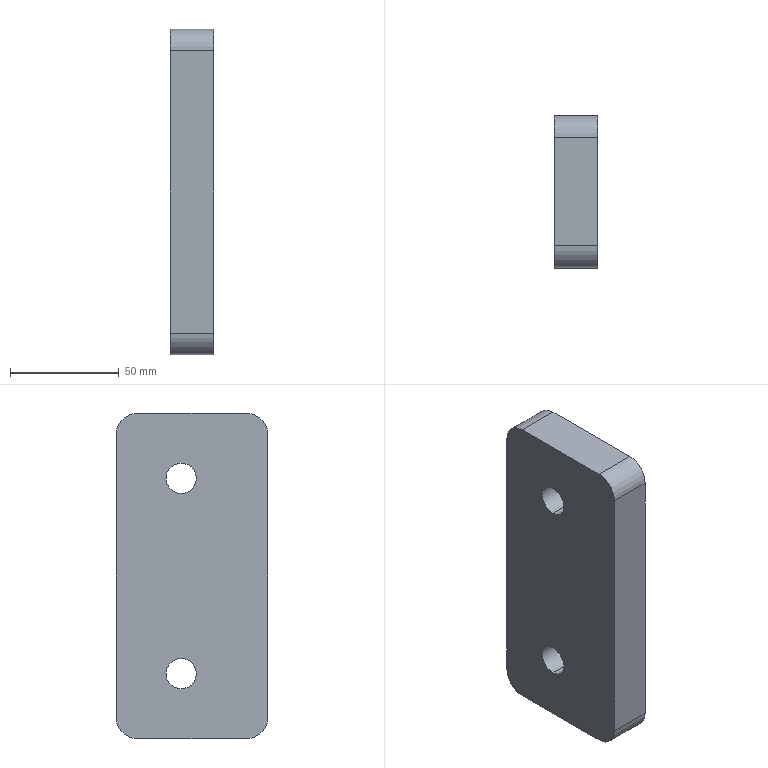Part | SolidWorks | 1 solid | 14 faces | box 20 x 70 x 150 mm | volume 202126 mm3 | cylinder 8 | plane 6 | commonest cylinder face diameters 14 x4 20 x4
STEP:
#1=CARTESIAN_POINT('',(-20.,5.,-38.));
#2=VERTEX_POINT('',#1);
#3=CARTESIAN_POINT('',(-20.,5.,-52.));
#4=VERTEX_POINT('',#3);
#5=CARTESIAN_POINT('',(-20.,5.,-45.));
#6=DIRECTION('',(-1.,0.,0.));
#7=DIRECTION('',(0.,0.,1.));
#8=AXIS2_PLACEMENT_3D('',#5,#6,#7);
#9=CIRCLE('',#8,7.);
#10=EDGE_CURVE('',#2,#4,#9,.T.);
#11=ORIENTED_EDGE('',*,*,#10,.T.);
#12=CARTESIAN_POINT('',(0.,5.,-52.));
#13=VERTEX_POINT('',#12);
#14=CARTESIAN_POINT('',(0.,5.,-52.));
#15=DIRECTION('',(1.,0.,0.));
#16=VECTOR('',#15,1000.);
#17=LINE('',#14,#16);
#18=EDGE_CURVE('',#4,#13,#17,.T.);
#19=ORIENTED_EDGE('',*,*,#18,.T.);
#20=CARTESIAN_POINT('',(0.,5.,-38.));
#21=VERTEX_POINT('',#20);
#22=CARTESIAN_POINT('',(0.,5.,-45.));
#23=DIRECTION('',(-1.,0.,0.));
#24=DIRECTION('',(0.,0.,1.));
#25=AXIS2_PLACEMENT_3D('',#22,#23,#24);
#26=CIRCLE('',#25,7.);
#27=EDGE_CURVE('',#21,#13,#26,.T.);
#28=ORIENTED_EDGE('',*,*,#27,.F.);
#29=CARTESIAN_POINT('',(0.,5.,-38.));
#30=DIRECTION('',(1.,0.,0.));
#31=VECTOR('',#30,1000.);
#32=LINE('',#29,#31);
#33=EDGE_CURVE('',#2,#21,#32,.T.);
#34=ORIENTED_EDGE('',*,*,#33,.F.);
#35=EDGE_LOOP('',(#11,#19,#28,#34));
#36=FACE_OUTER_BOUND('',#35,.T.);
#37=CARTESIAN_POINT('',(0.,5.,-45.));
#38=DIRECTION('',(1.,0.,0.));
#39=DIRECTION('',(0.,0.,1.));
#40=AXIS2_PLACEMENT_3D('',#37,#38,#39);
#41=CYLINDRICAL_SURFACE('',#40,7.);
#42=ADVANCED_FACE('',(#36),#41,.F.);
#43=CARTESIAN_POINT('',(-20.,5.,52.));
#44=VERTEX_POINT('',#43);
#45=CARTESIAN_POINT('',(-20.,5.,38.));
#46=VERTEX_POINT('',#45);
#47=CARTESIAN_POINT('',(-20.,5.,45.));
#48=DIRECTION('',(-1.,0.,0.));
#49=DIRECTION('',(0.,0.,1.));
#50=AXIS2_PLACEMENT_3D('',#47,#48,#49);
#51=CIRCLE('',#50,7.);
#52=EDGE_CURVE('',#44,#46,#51,.T.);
#53=ORIENTED_EDGE('',*,*,#52,.T.);
#54=CARTESIAN_POINT('',(0.,5.,38.));
#55=VERTEX_POINT('',#54);
#56=CARTESIAN_POINT('',(0.,5.,38.));
#57=DIRECTION('',(1.,0.,0.));
#58=VECTOR('',#57,1000.);
#59=LINE('',#56,#58);
#60=EDGE_CURVE('',#46,#55,#59,.T.);
#61=ORIENTED_EDGE('',*,*,#60,.T.);
#62=CARTESIAN_POINT('',(0.,5.,52.));
#63=VERTEX_POINT('',#62);
#64=CARTESIAN_POINT('',(0.,5.,45.));
#65=DIRECTION('',(-1.,0.,0.));
#66=DIRECTION('',(0.,0.,1.));
#67=AXIS2_PLACEMENT_3D('',#64,#65,#66);
#68=CIRCLE('',#67,7.);
#69=EDGE_CURVE('',#63,#55,#68,.T.);
#70=ORIENTED_EDGE('',*,*,#69,.F.);
#71=CARTESIAN_POINT('',(0.,5.,52.));
#72=DIRECTION('',(1.,0.,0.));
#73=VECTOR('',#72,1000.);
#74=LINE('',#71,#73);
#75=EDGE_CURVE('',#44,#63,#74,.T.);
#76=ORIENTED_EDGE('',*,*,#75,.F.);
#77=EDGE_LOOP('',(#53,#61,#70,#76));
#78=FACE_OUTER_BOUND('',#77,.T.);
#79=CARTESIAN_POINT('',(0.,5.,45.));
#80=DIRECTION('',(1.,0.,0.));
#81=DIRECTION('',(0.,0.,1.));
#82=AXIS2_PLACEMENT_3D('',#79,#80,#81);
#83=CYLINDRICAL_SURFACE('',#82,7.);
#84=ADVANCED_FACE('',(#78),#83,.F.);
#85=CARTESIAN_POINT('',(0.,25.,-75.));
#86=VERTEX_POINT('',#85);
#87=CARTESIAN_POINT('',(0.,-25.,-75.));
#88=VERTEX_POINT('',#87);
#89=CARTESIAN_POINT('',(0.,-35.,-75.));
#90=DIRECTION('',(0.,-1.,0.));
#91=VECTOR('',#90,1000.);
#92=LINE('',#89,#91);
#93=EDGE_CURVE('',#86,#88,#92,.T.);
#94=ORIENTED_EDGE('',*,*,#93,.T.);
#95=CARTESIAN_POINT('',(-20.,-25.,-75.));
#96=VERTEX_POINT('',#95);
#97=CARTESIAN_POINT('',(-20.,-25.,-75.));
#98=DIRECTION('',(1.,0.,0.));
#99=VECTOR('',#98,1000.);
#100=LINE('',#97,#99);
#101=EDGE_CURVE('',#96,#88,#100,.T.);
#102=ORIENTED_EDGE('',*,*,#101,.F.);
#103=CARTESIAN_POINT('',(-20.,25.,-75.));
#104=VERTEX_POINT('',#103);
#105=CARTESIAN_POINT('',(-20.,-35.,-75.));
#106=DIRECTION('',(0.,-1.,0.));
#107=VECTOR('',#106,1000.);
#108=LINE('',#105,#107);
#109=EDGE_CURVE('',#104,#96,#108,.T.);
#110=ORIENTED_EDGE('',*,*,#109,.F.);
#111=CARTESIAN_POINT('',(-20.,25.,-75.));
#112=DIRECTION('',(-1.,0.,0.));
#113=VECTOR('',#112,1000.);
#114=LINE('',#111,#113);
#115=EDGE_CURVE('',#86,#104,#114,.T.);
#116=ORIENTED_EDGE('',*,*,#115,.F.);
#117=EDGE_LOOP('',(#94,#102,#110,#116));
#118=FACE_OUTER_BOUND('',#117,.T.);
#119=CARTESIAN_POINT('',(-20.,-35.,-75.));
#120=DIRECTION('',(0.,0.,-1.));
#121=DIRECTION('',(1.,0.,0.));
#122=AXIS2_PLACEMENT_3D('',#119,#120,#121);
#123=PLANE('',#122);
#124=ADVANCED_FACE('',(#118),#123,.T.);
#125=CARTESIAN_POINT('',(0.,35.,65.));
#126=VERTEX_POINT('',#125);
#127=CARTESIAN_POINT('',(0.,35.,-65.));
#128=VERTEX_POINT('',#127);
#129=CARTESIAN_POINT('',(0.,35.,75.));
#130=DIRECTION('',(0.,0.,-1.));
#131=VECTOR('',#130,1000.);
#132=LINE('',#129,#131);
#133=EDGE_CURVE('',#126,#128,#132,.T.);
#134=ORIENTED_EDGE('',*,*,#133,.T.);
#135=CARTESIAN_POINT('',(-20.,35.,-65.));
#136=VERTEX_POINT('',#135);
#137=CARTESIAN_POINT('',(-20.,35.,-65.));
#138=DIRECTION('',(1.,0.,0.));
#139=VECTOR('',#138,1000.);
#140=LINE('',#137,#139);
#141=EDGE_CURVE('',#136,#128,#140,.T.);
#142=ORIENTED_EDGE('',*,*,#141,.F.);
#143=CARTESIAN_POINT('',(-20.,35.,65.));
#144=VERTEX_POINT('',#143);
#145=CARTESIAN_POINT('',(-20.,35.,75.));
#146=DIRECTION('',(0.,0.,-1.));
#147=VECTOR('',#146,1000.);
#148=LINE('',#145,#147);
#149=EDGE_CURVE('',#144,#136,#148,.T.);
#150=ORIENTED_EDGE('',*,*,#149,.F.);
#151=CARTESIAN_POINT('',(-20.,35.,65.));
#152=DIRECTION('',(-1.,0.,0.));
#153=VECTOR('',#152,1000.);
#154=LINE('',#151,#153);
#155=EDGE_CURVE('',#126,#144,#154,.T.);
#156=ORIENTED_EDGE('',*,*,#155,.F.);
#157=EDGE_LOOP('',(#134,#142,#150,#156));
#158=FACE_OUTER_BOUND('',#157,.T.);
#159=CARTESIAN_POINT('',(-20.,35.,75.));
#160=DIRECTION('',(0.,1.,0.));
#161=DIRECTION('',(0.,0.,-1.));
#162=AXIS2_PLACEMENT_3D('',#159,#160,#161);
#163=PLANE('',#162);
#164=ADVANCED_FACE('',(#158),#163,.T.);
#165=CARTESIAN_POINT('',(0.,-25.,75.));
#166=VERTEX_POINT('',#165);
#167=CARTESIAN_POINT('',(0.,25.,75.));
#168=VERTEX_POINT('',#167);
#169=CARTESIAN_POINT('',(0.,-35.,75.));
#170=DIRECTION('',(0.,1.,0.));
#171=VECTOR('',#170,1000.);
#172=LINE('',#169,#171);
#173=EDGE_CURVE('',#166,#168,#172,.T.);
#174=ORIENTED_EDGE('',*,*,#173,.T.);
#175=CARTESIAN_POINT('',(-20.,25.,75.));
#176=VERTEX_POINT('',#175);
#177=CARTESIAN_POINT('',(-20.,25.,75.));
#178=DIRECTION('',(1.,0.,0.));
#179=VECTOR('',#178,1000.);
#180=LINE('',#177,#179);
#181=EDGE_CURVE('',#176,#168,#180,.T.);
#182=ORIENTED_EDGE('',*,*,#181,.F.);
#183=CARTESIAN_POINT('',(-20.,-25.,75.));
#184=VERTEX_POINT('',#183);
#185=CARTESIAN_POINT('',(-20.,-35.,75.));
#186=DIRECTION('',(0.,1.,0.));
#187=VECTOR('',#186,1000.);
#188=LINE('',#185,#187);
#189=EDGE_CURVE('',#184,#176,#188,.T.);
#190=ORIENTED_EDGE('',*,*,#189,.F.);
#191=CARTESIAN_POINT('',(-20.,-25.,75.));
#192=DIRECTION('',(-1.,0.,0.));
#193=VECTOR('',#192,1000.);
#194=LINE('',#191,#193);
#195=EDGE_CURVE('',#166,#184,#194,.T.);
#196=ORIENTED_EDGE('',*,*,#195,.F.);
#197=EDGE_LOOP('',(#174,#182,#190,#196));
#198=FACE_OUTER_BOUND('',#197,.T.);
#199=CARTESIAN_POINT('',(-20.,-35.,75.));
#200=DIRECTION('',(0.,0.,1.));
#201=DIRECTION('',(-1.,0.,0.));
#202=AXIS2_PLACEMENT_3D('',#199,#200,#201);
#203=PLANE('',#202);
#204=ADVANCED_FACE('',(#198),#203,.T.);
#205=CARTESIAN_POINT('',(-20.,-35.,-65.));
#206=VERTEX_POINT('',#205);
#207=CARTESIAN_POINT('',(-20.,-35.,65.));
#208=VERTEX_POINT('',#207);
#209=CARTESIAN_POINT('',(-20.,-35.,75.));
#210=DIRECTION('',(0.,0.,1.));
#211=VECTOR('',#210,1000.);
#212=LINE('',#209,#211);
#213=EDGE_CURVE('',#206,#208,#212,.T.);
#214=ORIENTED_EDGE('',*,*,#213,.F.);
#215=CARTESIAN_POINT('',(0.,-35.,-65.));
#216=VERTEX_POINT('',#215);
#217=CARTESIAN_POINT('',(-20.,-35.,-65.));
#218=DIRECTION('',(-1.,0.,0.));
#219=VECTOR('',#218,1000.);
#220=LINE('',#217,#219);
#221=EDGE_CURVE('',#216,#206,#220,.T.);
#222=ORIENTED_EDGE('',*,*,#221,.F.);
#223=CARTESIAN_POINT('',(0.,-35.,65.));
#224=VERTEX_POINT('',#223);
#225=CARTESIAN_POINT('',(0.,-35.,75.));
#226=DIRECTION('',(0.,0.,1.));
#227=VECTOR('',#226,1000.);
#228=LINE('',#225,#227);
#229=EDGE_CURVE('',#216,#224,#228,.T.);
#230=ORIENTED_EDGE('',*,*,#229,.T.);
#231=CARTESIAN_POINT('',(-20.,-35.,65.));
#232=DIRECTION('',(1.,0.,0.));
#233=VECTOR('',#232,1000.);
#234=LINE('',#231,#233);
#235=EDGE_CURVE('',#208,#224,#234,.T.);
#236=ORIENTED_EDGE('',*,*,#235,.F.);
#237=EDGE_LOOP('',(#214,#222,#230,#236));
#238=FACE_OUTER_BOUND('',#237,.T.);
#239=CARTESIAN_POINT('',(-20.,-35.,75.));
#240=DIRECTION('',(0.,-1.,0.));
#241=DIRECTION('',(0.,0.,1.));
#242=AXIS2_PLACEMENT_3D('',#239,#240,#241);
#243=PLANE('',#242);
#244=ADVANCED_FACE('',(#238),#243,.T.);
#245=ORIENTED_EDGE('',*,*,#10,.F.);
#246=CARTESIAN_POINT('',(-20.,5.,-45.));
#247=DIRECTION('',(-1.,0.,0.));
#248=DIRECTION('',(0.,0.,1.));
#249=AXIS2_PLACEMENT_3D('',#246,#247,#248);
#250=CIRCLE('',#249,7.);
#251=EDGE_CURVE('',#4,#2,#250,.T.);
#252=ORIENTED_EDGE('',*,*,#251,.F.);
#253=EDGE_LOOP('',(#245,#252));
#254=FACE_BOUND('',#253,.T.);
#255=ORIENTED_EDGE('',*,*,#52,.F.);
#256=CARTESIAN_POINT('',(-20.,5.,45.));
#257=DIRECTION('',(-1.,0.,0.));
#258=DIRECTION('',(0.,0.,1.));
#259=AXIS2_PLACEMENT_3D('',#256,#257,#258);
#260=CIRCLE('',#259,7.);
#261=EDGE_CURVE('',#46,#44,#260,.T.);
#262=ORIENTED_EDGE('',*,*,#261,.F.);
#263=EDGE_LOOP('',(#255,#262));
#264=FACE_BOUND('',#263,.T.);
#265=ORIENTED_EDGE('',*,*,#189,.T.);
#266=CARTESIAN_POINT('',(-20.,25.,65.));
#267=DIRECTION('',(1.,0.,0.));
#268=DIRECTION('',(0.,0.,1.));
#269=AXIS2_PLACEMENT_3D('',#266,#267,#268);
#270=CIRCLE('',#269,10.);
#271=EDGE_CURVE('',#144,#176,#270,.T.);
#272=ORIENTED_EDGE('',*,*,#271,.F.);
#273=ORIENTED_EDGE('',*,*,#149,.T.);
#274=CARTESIAN_POINT('',(-20.,25.,-65.));
#275=DIRECTION('',(1.,0.,0.));
#276=DIRECTION('',(0.,0.,1.));
#277=AXIS2_PLACEMENT_3D('',#274,#275,#276);
#278=CIRCLE('',#277,10.);
#279=EDGE_CURVE('',#104,#136,#278,.T.);
#280=ORIENTED_EDGE('',*,*,#279,.F.);
#281=ORIENTED_EDGE('',*,*,#109,.T.);
#282=CARTESIAN_POINT('',(-20.,-25.,-65.));
#283=DIRECTION('',(1.,0.,0.));
#284=DIRECTION('',(0.,0.,1.));
#285=AXIS2_PLACEMENT_3D('',#282,#283,#284);
#286=CIRCLE('',#285,10.);
#287=EDGE_CURVE('',#206,#96,#286,.T.);
#288=ORIENTED_EDGE('',*,*,#287,.F.);
#289=ORIENTED_EDGE('',*,*,#213,.T.);
#290=CARTESIAN_POINT('',(-20.,-25.,65.));
#291=DIRECTION('',(1.,0.,0.));
#292=DIRECTION('',(0.,0.,1.));
#293=AXIS2_PLACEMENT_3D('',#290,#291,#292);
#294=CIRCLE('',#293,10.);
#295=EDGE_CURVE('',#184,#208,#294,.T.);
#296=ORIENTED_EDGE('',*,*,#295,.F.);
#297=EDGE_LOOP('',(#265,#272,#273,#280,#281,#288,#289,#296));
#298=FACE_OUTER_BOUND('',#297,.T.);
#299=CARTESIAN_POINT('',(-20.,0.,0.));
#300=DIRECTION('',(1.,0.,0.));
#301=DIRECTION('',(0.,0.,1.));
#302=AXIS2_PLACEMENT_3D('',#299,#300,#301);
#303=PLANE('',#302);
#304=ADVANCED_FACE('',(#254,#264,#298),#303,.F.);
#305=ORIENTED_EDGE('',*,*,#27,.T.);
#306=CARTESIAN_POINT('',(0.,5.,-45.));
#307=DIRECTION('',(-1.,0.,0.));
#308=DIRECTION('',(0.,0.,1.));
#309=AXIS2_PLACEMENT_3D('',#306,#307,#308);
#310=CIRCLE('',#309,7.);
#311=EDGE_CURVE('',#13,#21,#310,.T.);
#312=ORIENTED_EDGE('',*,*,#311,.T.);
#313=EDGE_LOOP('',(#305,#312));
#314=FACE_BOUND('',#313,.T.);
#315=ORIENTED_EDGE('',*,*,#69,.T.);
#316=CARTESIAN_POINT('',(0.,5.,45.));
#317=DIRECTION('',(-1.,0.,0.));
#318=DIRECTION('',(0.,0.,1.));
#319=AXIS2_PLACEMENT_3D('',#316,#317,#318);
#320=CIRCLE('',#319,7.);
#321=EDGE_CURVE('',#55,#63,#320,.T.);
#322=ORIENTED_EDGE('',*,*,#321,.T.);
#323=EDGE_LOOP('',(#315,#322));
#324=FACE_BOUND('',#323,.T.);
#325=ORIENTED_EDGE('',*,*,#229,.F.);
#326=CARTESIAN_POINT('',(0.,-25.,-65.));
#327=DIRECTION('',(-1.,0.,0.));
#328=DIRECTION('',(0.,0.,1.));
#329=AXIS2_PLACEMENT_3D('',#326,#327,#328);
#330=CIRCLE('',#329,10.);
#331=EDGE_CURVE('',#88,#216,#330,.T.);
#332=ORIENTED_EDGE('',*,*,#331,.F.);
#333=ORIENTED_EDGE('',*,*,#93,.F.);
#334=CARTESIAN_POINT('',(0.,25.,-65.));
#335=DIRECTION('',(-1.,0.,0.));
#336=DIRECTION('',(0.,0.,1.));
#337=AXIS2_PLACEMENT_3D('',#334,#335,#336);
#338=CIRCLE('',#337,10.);
#339=EDGE_CURVE('',#128,#86,#338,.T.);
#340=ORIENTED_EDGE('',*,*,#339,.F.);
#341=ORIENTED_EDGE('',*,*,#133,.F.);
#342=CARTESIAN_POINT('',(0.,25.,65.));
#343=DIRECTION('',(-1.,0.,0.));
#344=DIRECTION('',(0.,0.,1.));
#345=AXIS2_PLACEMENT_3D('',#342,#343,#344);
#346=CIRCLE('',#345,10.);
#347=EDGE_CURVE('',#168,#126,#346,.T.);
#348=ORIENTED_EDGE('',*,*,#347,.F.);
#349=ORIENTED_EDGE('',*,*,#173,.F.);
#350=CARTESIAN_POINT('',(0.,-25.,65.));
#351=DIRECTION('',(-1.,0.,0.));
#352=DIRECTION('',(0.,0.,1.));
#353=AXIS2_PLACEMENT_3D('',#350,#351,#352);
#354=CIRCLE('',#353,10.);
#355=EDGE_CURVE('',#224,#166,#354,.T.);
#356=ORIENTED_EDGE('',*,*,#355,.F.);
#357=EDGE_LOOP('',(#325,#332,#333,#340,#341,#348,#349,#356));
#358=FACE_OUTER_BOUND('',#357,.T.);
#359=CARTESIAN_POINT('',(0.,0.,0.));
#360=DIRECTION('',(1.,0.,0.));
#361=DIRECTION('',(0.,0.,1.));
#362=AXIS2_PLACEMENT_3D('',#359,#360,#361);
#363=PLANE('',#362);
#364=ADVANCED_FACE('',(#314,#324,#358),#363,.T.);
#365=ORIENTED_EDGE('',*,*,#60,.F.);
#366=ORIENTED_EDGE('',*,*,#261,.T.);
#367=ORIENTED_EDGE('',*,*,#75,.T.);
#368=ORIENTED_EDGE('',*,*,#321,.F.);
#369=EDGE_LOOP('',(#365,#366,#367,#368));
#370=FACE_OUTER_BOUND('',#369,.T.);
#371=CARTESIAN_POINT('',(0.,5.,45.));
#372=DIRECTION('',(1.,0.,0.));
#373=DIRECTION('',(0.,0.,1.));
#374=AXIS2_PLACEMENT_3D('',#371,#372,#373);
#375=CYLINDRICAL_SURFACE('',#374,7.);
#376=ADVANCED_FACE('',(#370),#375,.F.);
#377=ORIENTED_EDGE('',*,*,#18,.F.);
#378=ORIENTED_EDGE('',*,*,#251,.T.);
#379=ORIENTED_EDGE('',*,*,#33,.T.);
#380=ORIENTED_EDGE('',*,*,#311,.F.);
#381=EDGE_LOOP('',(#377,#378,#379,#380));
#382=FACE_OUTER_BOUND('',#381,.T.);
#383=CARTESIAN_POINT('',(0.,5.,-45.));
#384=DIRECTION('',(1.,0.,0.));
#385=DIRECTION('',(0.,0.,1.));
#386=AXIS2_PLACEMENT_3D('',#383,#384,#385);
#387=CYLINDRICAL_SURFACE('',#386,7.);
#388=ADVANCED_FACE('',(#382),#387,.F.);
#389=ORIENTED_EDGE('',*,*,#295,.T.);
#390=ORIENTED_EDGE('',*,*,#235,.T.);
#391=ORIENTED_EDGE('',*,*,#355,.T.);
#392=ORIENTED_EDGE('',*,*,#195,.T.);
#393=EDGE_LOOP('',(#389,#390,#391,#392));
#394=FACE_OUTER_BOUND('',#393,.T.);
#395=CARTESIAN_POINT('',(-20.,-25.,65.));
#396=DIRECTION('',(1.,0.,0.));
#397=DIRECTION('',(0.,0.,1.));
#398=AXIS2_PLACEMENT_3D('',#395,#396,#397);
#399=CYLINDRICAL_SURFACE('',#398,10.);
#400=ADVANCED_FACE('',(#394),#399,.T.);
#401=ORIENTED_EDGE('',*,*,#271,.T.);
#402=ORIENTED_EDGE('',*,*,#181,.T.);
#403=ORIENTED_EDGE('',*,*,#347,.T.);
#404=ORIENTED_EDGE('',*,*,#155,.T.);
#405=EDGE_LOOP('',(#401,#402,#403,#404));
#406=FACE_OUTER_BOUND('',#405,.T.);
#407=CARTESIAN_POINT('',(-20.,25.,65.));
#408=DIRECTION('',(1.,0.,0.));
#409=DIRECTION('',(0.,0.,1.));
#410=AXIS2_PLACEMENT_3D('',#407,#408,#409);
#411=CYLINDRICAL_SURFACE('',#410,10.);
#412=ADVANCED_FACE('',(#406),#411,.T.);
#413=ORIENTED_EDGE('',*,*,#279,.T.);
#414=ORIENTED_EDGE('',*,*,#141,.T.);
#415=ORIENTED_EDGE('',*,*,#339,.T.);
#416=ORIENTED_EDGE('',*,*,#115,.T.);
#417=EDGE_LOOP('',(#413,#414,#415,#416));
#418=FACE_OUTER_BOUND('',#417,.T.);
#419=CARTESIAN_POINT('',(-20.,25.,-65.));
#420=DIRECTION('',(1.,0.,0.));
#421=DIRECTION('',(0.,0.,1.));
#422=AXIS2_PLACEMENT_3D('',#419,#420,#421);
#423=CYLINDRICAL_SURFACE('',#422,10.);
#424=ADVANCED_FACE('',(#418),#423,.T.);
#425=ORIENTED_EDGE('',*,*,#287,.T.);
#426=ORIENTED_EDGE('',*,*,#101,.T.);
#427=ORIENTED_EDGE('',*,*,#331,.T.);
#428=ORIENTED_EDGE('',*,*,#221,.T.);
#429=EDGE_LOOP('',(#425,#426,#427,#428));
#430=FACE_OUTER_BOUND('',#429,.T.);
#431=CARTESIAN_POINT('',(-20.,-25.,-65.));
#432=DIRECTION('',(1.,0.,0.));
#433=DIRECTION('',(0.,0.,1.));
#434=AXIS2_PLACEMENT_3D('',#431,#432,#433);
#435=CYLINDRICAL_SURFACE('',#434,10.);
#436=ADVANCED_FACE('',(#430),#435,.T.);
#437=CLOSED_SHELL('',(#42,#84,#124,#164,#204,#244,#304,#364,#376,#388,#400,#412,#424,#436));
#438=MANIFOLD_SOLID_BREP('',#437);
#439=CARTESIAN_POINT('',(0.,0.,0.));
#440=DIRECTION('',(0.,0.,1.));
#441=DIRECTION('',(1.,0.,0.));
#442=AXIS2_PLACEMENT_3D('',#439,#440,#441);
#443=(LENGTH_UNIT()NAMED_UNIT(*)SI_UNIT(.MILLI.,.METRE.));
#444=UNCERTAINTY_MEASURE_WITH_UNIT(LENGTH_MEASURE(0.00001),#443,'','');
#445=(NAMED_UNIT(*)PLANE_ANGLE_UNIT()SI_UNIT($,.RADIAN.));
#446=(NAMED_UNIT(*)SI_UNIT($,.STERADIAN.)SOLID_ANGLE_UNIT());
#447=(GEOMETRIC_REPRESENTATION_CONTEXT(3)GLOBAL_UNCERTAINTY_ASSIGNED_CONTEXT((#444))GLOBAL_UNIT_ASSIGNED_CONTEXT((#443,#445,#446))REPRESENTATION_CONTEXT('',''));
#448=ADVANCED_BREP_SHAPE_REPRESENTATION('',(#438,#442),#447);